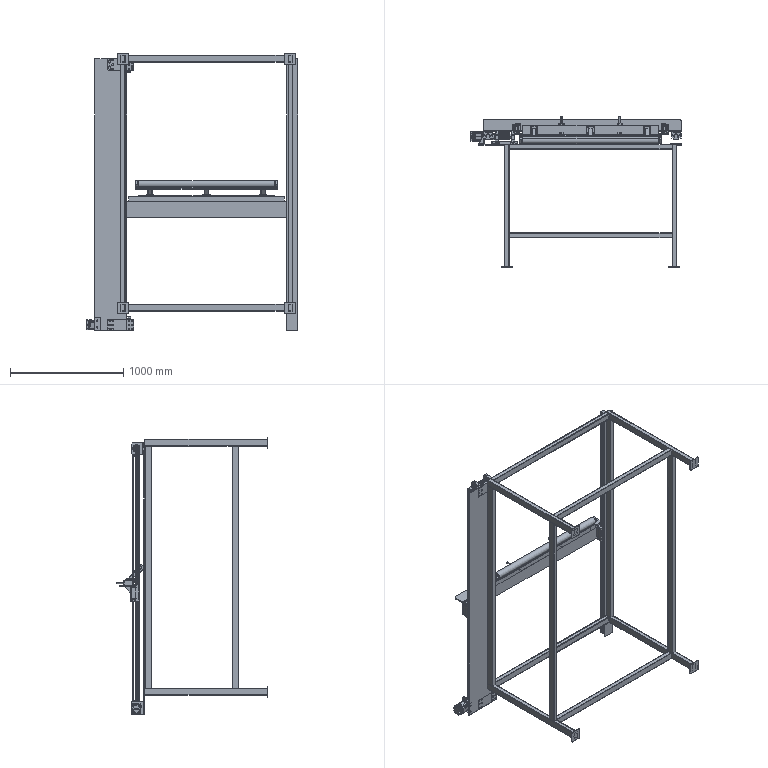Part | SolidWorks | features CompositeCurve 8, Belt 1, InContextFeatHolder 1 | 78 solids | 6573 faces | volume 35795724 mm3 | plane 2777 | cylinder 2613 | spline 681 | cone 502 | commonest cylinder face diameters 1 x249 0.2 x153 1.5 x124 0.8 x121 20 x119 4 x110